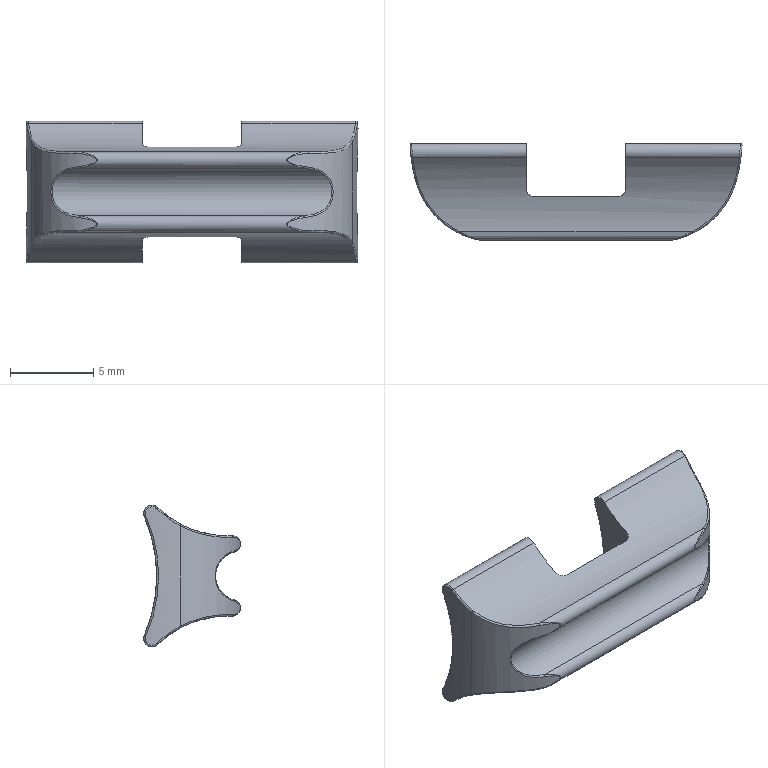Part | STEP file | PRT0001_68_27 | 1 solid | 59 faces | box 19.974 x 5.821 x 8.525 mm | volume 410.28 mm3 | spline 31 | cylinder 25 | plane 3 | commonest cylinder face diameters 1 x16 10 x2 11.88 x2 17.8 x2 20 x2 2.981 x1